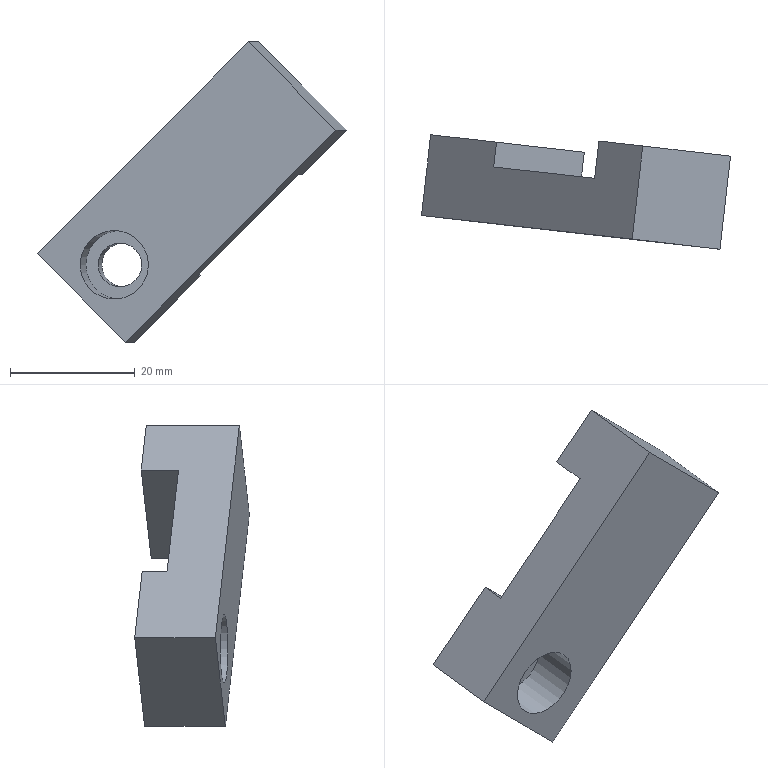Part | NX | features XQ 2 | 1 solid | 13 faces | box 49.472 x 18.36 x 48.083 mm | volume 10087 mm3 | plane 11 | cylinder 2 | commonest cylinder face diameters 7 x1 11 x1
STEP:
#1=CARTESIAN_POINT('',(2718.933,-373.251,-72.883));
#2=VERTEX_POINT('',#1);
#3=CARTESIAN_POINT('',(2735.092,-375.092,-56.62));
#4=VERTEX_POINT('',#3);
#5=CARTESIAN_POINT('',(2735.092,-375.092,-56.62));
#6=DIRECTION('',(0.7026,-0.08005,0.7071));
#7=VECTOR('',#6,1000.);
#8=LINE('',#5,#7);
#9=EDGE_CURVE('',#2,#4,#8,.T.);
#10=ORIENTED_EDGE('',*,*,#9,.F.);
#11=CARTESIAN_POINT('',(2704.882,-371.65,-58.741));
#12=VERTEX_POINT('',#11);
#13=CARTESIAN_POINT('',(2711.907,-372.45,-65.812));
#14=DIRECTION('',(-0.7026,0.08005,0.7071));
#15=VECTOR('',#14,1000.);
#16=LINE('',#13,#15);
#17=EDGE_CURVE('',#2,#12,#16,.T.);
#18=ORIENTED_EDGE('',*,*,#17,.T.);
#19=CARTESIAN_POINT('',(2721.041,-373.491,-42.478));
#20=VERTEX_POINT('',#19);
#21=CARTESIAN_POINT('',(2721.041,-373.491,-42.478));
#22=DIRECTION('',(-0.7026,0.08005,-0.7071));
#23=VECTOR('',#22,1000.);
#24=LINE('',#21,#23);
#25=EDGE_CURVE('',#20,#12,#24,.T.);
#26=ORIENTED_EDGE('',*,*,#25,.F.);
#27=CARTESIAN_POINT('',(2728.066,-374.292,-49.549));
#28=DIRECTION('',(0.7026,-0.08005,-0.7071));
#29=VECTOR('',#28,1000.);
#30=LINE('',#27,#29);
#31=EDGE_CURVE('',#20,#4,#30,.T.);
#32=ORIENTED_EDGE('',*,*,#31,.T.);
#33=EDGE_LOOP('',(#10,#18,#26,#32));
#34=FACE_BOUND('',#33,.T.);
#35=CARTESIAN_POINT('',(2737.38,-375.353,-28.774));
#36=DIRECTION('',(0.1132,0.9936,-0.000000218));
#37=DIRECTION('',(-0.000000616,-0.000000149,-1.));
#38=AXIS2_PLACEMENT_3D('',#35,#36,#37);
#39=PLANE('',#38);
#40=ADVANCED_FACE('',(#34),#39,.T.);
#41=CARTESIAN_POINT('',(2694.796,-366.475,-69.348));
#42=VERTEX_POINT('',#41);
#43=CARTESIAN_POINT('',(2693.325,-379.391,-69.348));
#44=VERTEX_POINT('',#43);
#45=CARTESIAN_POINT('',(2694.457,-369.456,-69.348));
#46=DIRECTION('',(-0.1132,-0.9936,0.000000275));
#47=VECTOR('',#46,1000.);
#48=LINE('',#45,#47);
#49=EDGE_CURVE('',#42,#44,#48,.T.);
#50=ORIENTED_EDGE('',*,*,#49,.F.);
#51=CARTESIAN_POINT('',(2708.847,-368.076,-83.49));
#52=VERTEX_POINT('',#51);
#53=CARTESIAN_POINT('',(2703.578,-367.476,-78.187));
#54=DIRECTION('',(-0.7026,0.08005,0.7071));
#55=VECTOR('',#54,1000.);
#56=LINE('',#53,#55);
#57=EDGE_CURVE('',#52,#42,#56,.T.);
#58=ORIENTED_EDGE('',*,*,#57,.F.);
#59=CARTESIAN_POINT('',(2707.376,-380.992,-83.49));
#60=VERTEX_POINT('',#59);
#61=CARTESIAN_POINT('',(2708.508,-371.057,-83.49));
#62=DIRECTION('',(0.1132,0.9936,-0.000000275));
#63=VECTOR('',#62,1000.);
#64=LINE('',#61,#63);
#65=EDGE_CURVE('',#60,#52,#64,.T.);
#66=ORIENTED_EDGE('',*,*,#65,.F.);
#67=CARTESIAN_POINT('',(2702.107,-380.392,-78.187));
#68=DIRECTION('',(0.7026,-0.08005,-0.7071));
#69=VECTOR('',#68,1000.);
#70=LINE('',#67,#69);
#71=EDGE_CURVE('',#44,#60,#70,.T.);
#72=ORIENTED_EDGE('',*,*,#71,.F.);
#73=EDGE_LOOP('',(#50,#58,#66,#72));
#74=FACE_BOUND('',#73,.T.);
#75=CARTESIAN_POINT('',(2703.239,-370.456,-78.187));
#76=DIRECTION('',(-0.7026,0.08005,-0.7071));
#77=DIRECTION('',(0.7112,0.0435,-0.7017));
#78=AXIS2_PLACEMENT_3D('',#75,#76,#77);
#79=PLANE('',#78);
#80=ADVANCED_FACE('',(#74),#79,.T.);
#81=ORIENTED_EDGE('',*,*,#25,.T.);
#82=CARTESIAN_POINT('',(2705.335,-367.676,-58.741));
#83=VERTEX_POINT('',#82);
#84=CARTESIAN_POINT('',(2704.995,-370.656,-58.741));
#85=DIRECTION('',(0.1132,0.9936,-0.000000275));
#86=VECTOR('',#85,1000.);
#87=LINE('',#84,#86);
#88=EDGE_CURVE('',#12,#83,#87,.T.);
#89=ORIENTED_EDGE('',*,*,#88,.T.);
#90=CARTESIAN_POINT('',(2721.493,-369.517,-42.478));
#91=DIRECTION('',(-0.7026,0.08005,-0.7071));
#92=VECTOR('',#91,1000.);
#93=LINE('',#90,#92);
#94=EDGE_CURVE('',#83,#42,#93,.T.);
#95=ORIENTED_EDGE('',*,*,#94,.T.);
#96=ORIENTED_EDGE('',*,*,#49,.T.);
#97=CARTESIAN_POINT('',(2727.047,-383.234,-35.407));
#98=VERTEX_POINT('',#97);
#99=CARTESIAN_POINT('',(2720.022,-382.433,-42.478));
#100=DIRECTION('',(-0.7026,0.08005,-0.7071));
#101=VECTOR('',#100,1000.);
#102=LINE('',#99,#101);
#103=EDGE_CURVE('',#98,#44,#102,.T.);
#104=ORIENTED_EDGE('',*,*,#103,.F.);
#105=CARTESIAN_POINT('',(2728.745,-368.33,-35.407));
#106=VERTEX_POINT('',#105);
#107=CARTESIAN_POINT('',(2728.179,-373.298,-35.407));
#108=DIRECTION('',(0.1132,0.9936,-0.000000275));
#109=VECTOR('',#108,1000.);
#110=LINE('',#107,#109);
#111=EDGE_CURVE('',#98,#106,#110,.T.);
#112=ORIENTED_EDGE('',*,*,#111,.T.);
#113=CARTESIAN_POINT('',(2721.72,-367.53,-42.478));
#114=VERTEX_POINT('',#113);
#115=CARTESIAN_POINT('',(2714.694,-366.729,-49.549));
#116=DIRECTION('',(-0.7026,0.08005,-0.7071));
#117=VECTOR('',#116,1000.);
#118=LINE('',#115,#117);
#119=EDGE_CURVE('',#106,#114,#118,.T.);
#120=ORIENTED_EDGE('',*,*,#119,.T.);
#121=CARTESIAN_POINT('',(2721.154,-372.498,-42.478));
#122=DIRECTION('',(0.1132,0.9936,-0.000000275));
#123=VECTOR('',#122,1000.);
#124=LINE('',#121,#123);
#125=EDGE_CURVE('',#20,#114,#124,.T.);
#126=ORIENTED_EDGE('',*,*,#125,.F.);
#127=EDGE_LOOP('',(#81,#89,#95,#96,#104,#112,#120,#126));
#128=FACE_BOUND('',#127,.T.);
#129=CARTESIAN_POINT('',(2721.154,-372.498,-42.478));
#130=DIRECTION('',(-0.7026,0.08005,0.7071));
#131=DIRECTION('',(-0.6832,0.2024,-0.7017));
#132=AXIS2_PLACEMENT_3D('',#129,#130,#131);
#133=PLANE('',#132);
#134=ADVANCED_FACE('',(#128),#133,.T.);
#135=ORIENTED_EDGE('',*,*,#9,.T.);
#136=CARTESIAN_POINT('',(2735.771,-369.131,-56.62));
#137=VERTEX_POINT('',#136);
#138=CARTESIAN_POINT('',(2735.205,-374.098,-56.62));
#139=DIRECTION('',(0.1132,0.9936,-0.000000275));
#140=VECTOR('',#139,1000.);
#141=LINE('',#138,#140);
#142=EDGE_CURVE('',#4,#137,#141,.T.);
#143=ORIENTED_EDGE('',*,*,#142,.T.);
#144=CARTESIAN_POINT('',(2742.797,-369.931,-49.549));
#145=VERTEX_POINT('',#144);
#146=CARTESIAN_POINT('',(2728.745,-368.33,-63.691));
#147=DIRECTION('',(-0.7026,0.08005,-0.7071));
#148=VECTOR('',#147,1000.);
#149=LINE('',#146,#148);
#150=EDGE_CURVE('',#145,#137,#149,.T.);
#151=ORIENTED_EDGE('',*,*,#150,.F.);
#152=CARTESIAN_POINT('',(2741.099,-384.835,-49.549));
#153=VERTEX_POINT('',#152);
#154=CARTESIAN_POINT('',(2742.231,-374.899,-49.549));
#155=DIRECTION('',(-0.1132,-0.9936,0.000000275));
#156=VECTOR('',#155,1000.);
#157=LINE('',#154,#156);
#158=EDGE_CURVE('',#145,#153,#157,.T.);
#159=ORIENTED_EDGE('',*,*,#158,.T.);
#160=CARTESIAN_POINT('',(2734.073,-384.034,-56.62));
#161=DIRECTION('',(-0.7026,0.08005,-0.7071));
#162=VECTOR('',#161,1000.);
#163=LINE('',#160,#162);
#164=EDGE_CURVE('',#153,#60,#163,.T.);
#165=ORIENTED_EDGE('',*,*,#164,.T.);
#166=ORIENTED_EDGE('',*,*,#65,.T.);
#167=CARTESIAN_POINT('',(2719.386,-369.277,-72.883));
#168=VERTEX_POINT('',#167);
#169=CARTESIAN_POINT('',(2735.545,-371.118,-56.62));
#170=DIRECTION('',(-0.7026,0.08005,-0.7071));
#171=VECTOR('',#170,1000.);
#172=LINE('',#169,#171);
#173=EDGE_CURVE('',#168,#52,#172,.T.);
#174=ORIENTED_EDGE('',*,*,#173,.F.);
#175=CARTESIAN_POINT('',(2719.046,-372.257,-72.883));
#176=DIRECTION('',(0.1132,0.9936,-0.000000275));
#177=VECTOR('',#176,1000.);
#178=LINE('',#175,#177);
#179=EDGE_CURVE('',#2,#168,#178,.T.);
#180=ORIENTED_EDGE('',*,*,#179,.F.);
#181=EDGE_LOOP('',(#135,#143,#151,#159,#165,#166,#174,#180));
#182=FACE_BOUND('',#181,.T.);
#183=CARTESIAN_POINT('',(2735.205,-374.098,-56.62));
#184=DIRECTION('',(0.7026,-0.08005,-0.7071));
#185=DIRECTION('',(0.6832,-0.2024,0.7017));
#186=AXIS2_PLACEMENT_3D('',#183,#184,#185);
#187=PLANE('',#186);
#188=ADVANCED_FACE('',(#182),#187,.T.);
#189=ORIENTED_EDGE('',*,*,#158,.F.);
#190=CARTESIAN_POINT('',(2737.527,-369.331,-44.246));
#191=DIRECTION('',(0.7026,-0.08005,-0.7071));
#192=VECTOR('',#191,1000.);
#193=LINE('',#190,#192);
#194=EDGE_CURVE('',#106,#145,#193,.T.);
#195=ORIENTED_EDGE('',*,*,#194,.F.);
#196=ORIENTED_EDGE('',*,*,#111,.F.);
#197=CARTESIAN_POINT('',(2735.829,-384.234,-44.246));
#198=DIRECTION('',(-0.7026,0.08005,0.7071));
#199=VECTOR('',#198,1000.);
#200=LINE('',#197,#199);
#201=EDGE_CURVE('',#153,#98,#200,.T.);
#202=ORIENTED_EDGE('',*,*,#201,.F.);
#203=EDGE_LOOP('',(#189,#195,#196,#202));
#204=FACE_BOUND('',#203,.T.);
#205=CARTESIAN_POINT('',(2736.961,-374.299,-44.246));
#206=DIRECTION('',(0.7026,-0.08005,0.7071));
#207=DIRECTION('',(-0.7112,-0.0435,0.7017));
#208=AXIS2_PLACEMENT_3D('',#205,#206,#207);
#209=PLANE('',#208);
#210=ADVANCED_FACE('',(#204),#209,.T.);
#211=ORIENTED_EDGE('',*,*,#103,.T.);
#212=ORIENTED_EDGE('',*,*,#71,.T.);
#213=ORIENTED_EDGE('',*,*,#164,.F.);
#214=ORIENTED_EDGE('',*,*,#201,.T.);
#215=EDGE_LOOP('',(#211,#212,#213,#214));
#216=FACE_BOUND('',#215,.T.);
#217=CARTESIAN_POINT('',(2711.084,-381.415,-71.116));
#218=VERTEX_POINT('',#217);
#219=CARTESIAN_POINT('',(2705.619,-380.792,-71.116));
#220=DIRECTION('',(0.1132,0.9936,-0.000000275));
#221=DIRECTION('',(0.9936,-0.1132,0.));
#222=AXIS2_PLACEMENT_3D('',#219,#220,#221);
#223=CIRCLE('',#222,5.5);
#224=EDGE_CURVE('',#218,#218,#223,.T.);
#225=ORIENTED_EDGE('',*,*,#224,.T.);
#226=EDGE_LOOP('',(#225));
#227=FACE_BOUND('',#226,.T.);
#228=CARTESIAN_POINT('',(2725.291,-383.034,-47.781));
#229=DIRECTION('',(-0.1132,-0.9936,0.000000275));
#230=DIRECTION('',(0.000000623,0.000000206,1.));
#231=AXIS2_PLACEMENT_3D('',#228,#229,#230);
#232=PLANE('',#231);
#233=ADVANCED_FACE('',(#216,#227),#232,.T.);
#234=CARTESIAN_POINT('',(2711.99,-373.466,-71.116));
#235=VERTEX_POINT('',#234);
#236=CARTESIAN_POINT('',(2706.525,-372.844,-71.116));
#237=DIRECTION('',(0.1132,0.9936,-0.000000275));
#238=DIRECTION('',(0.9936,-0.1132,0.));
#239=AXIS2_PLACEMENT_3D('',#236,#237,#238);
#240=CIRCLE('',#239,5.5);
#241=EDGE_CURVE('',#235,#235,#240,.T.);
#242=ORIENTED_EDGE('',*,*,#241,.T.);
#243=EDGE_LOOP('',(#242));
#244=FACE_BOUND('',#243,.T.);
#245=ORIENTED_EDGE('',*,*,#224,.F.);
#246=EDGE_LOOP('',(#245));
#247=FACE_BOUND('',#246,.T.);
#248=CARTESIAN_POINT('',(2706.185,-375.824,-71.116));
#249=DIRECTION('',(0.1132,0.9936,-0.000000275));
#250=DIRECTION('',(0.1725,-0.01966,-0.9848));
#251=AXIS2_PLACEMENT_3D('',#248,#249,#250);
#252=CYLINDRICAL_SURFACE('',#251,5.5);
#253=ADVANCED_FACE('',(#244,#247),#252,.F.);
#254=CARTESIAN_POINT('',(2710.002,-373.24,-71.116));
#255=VERTEX_POINT('',#254);
#256=CARTESIAN_POINT('',(2706.525,-372.844,-71.116));
#257=DIRECTION('',(-0.1132,-0.9936,0.000000275));
#258=DIRECTION('',(0.9936,-0.1132,0.));
#259=AXIS2_PLACEMENT_3D('',#256,#257,#258);
#260=CIRCLE('',#259,3.5);
#261=EDGE_CURVE('',#255,#255,#260,.T.);
#262=ORIENTED_EDGE('',*,*,#261,.F.);
#263=EDGE_LOOP('',(#262));
#264=FACE_BOUND('',#263,.T.);
#265=ORIENTED_EDGE('',*,*,#241,.F.);
#266=EDGE_LOOP('',(#265));
#267=FACE_BOUND('',#266,.T.);
#268=CARTESIAN_POINT('',(2706.525,-372.844,-71.116));
#269=DIRECTION('',(-0.1132,-0.9936,0.000000275));
#270=DIRECTION('',(0.000000623,0.000000206,1.));
#271=AXIS2_PLACEMENT_3D('',#268,#269,#270);
#272=PLANE('',#271);
#273=ADVANCED_FACE('',(#264,#267),#272,.T.);
#274=ORIENTED_EDGE('',*,*,#17,.F.);
#275=ORIENTED_EDGE('',*,*,#179,.T.);
#276=CARTESIAN_POINT('',(2712.36,-368.476,-65.812));
#277=DIRECTION('',(-0.7026,0.08005,0.7071));
#278=VECTOR('',#277,1000.);
#279=LINE('',#276,#278);
#280=EDGE_CURVE('',#168,#83,#279,.T.);
#281=ORIENTED_EDGE('',*,*,#280,.T.);
#282=ORIENTED_EDGE('',*,*,#88,.F.);
#283=EDGE_LOOP('',(#274,#275,#281,#282));
#284=FACE_BOUND('',#283,.T.);
#285=CARTESIAN_POINT('',(2712.021,-371.457,-65.812));
#286=DIRECTION('',(0.7026,-0.08005,0.7071));
#287=DIRECTION('',(-0.7112,-0.0435,0.7017));
#288=AXIS2_PLACEMENT_3D('',#285,#286,#287);
#289=PLANE('',#288);
#290=ADVANCED_FACE('',(#284),#289,.T.);
#291=CARTESIAN_POINT('',(2703.613,-367.48,-71.116));
#292=VERTEX_POINT('',#291);
#293=CARTESIAN_POINT('',(2707.091,-367.876,-71.116));
#294=DIRECTION('',(0.1132,0.9936,-0.000000275));
#295=DIRECTION('',(-0.9936,0.1132,0.));
#296=AXIS2_PLACEMENT_3D('',#293,#294,#295);
#297=CIRCLE('',#296,3.5);
#298=EDGE_CURVE('',#292,#292,#297,.T.);
#299=ORIENTED_EDGE('',*,*,#298,.F.);
#300=EDGE_LOOP('',(#299));
#301=FACE_BOUND('',#300,.T.);
#302=ORIENTED_EDGE('',*,*,#94,.F.);
#303=ORIENTED_EDGE('',*,*,#280,.F.);
#304=ORIENTED_EDGE('',*,*,#173,.T.);
#305=ORIENTED_EDGE('',*,*,#57,.T.);
#306=EDGE_LOOP('',(#302,#303,#304,#305));
#307=FACE_BOUND('',#306,.T.);
#308=CARTESIAN_POINT('',(2730.275,-370.517,-51.317));
#309=DIRECTION('',(0.1132,0.9936,-0.000000275));
#310=DIRECTION('',(-0.000000623,-0.000000206,-1.));
#311=AXIS2_PLACEMENT_3D('',#308,#309,#310);
#312=PLANE('',#311);
#313=ADVANCED_FACE('',(#301,#307),#312,.T.);
#314=ORIENTED_EDGE('',*,*,#298,.T.);
#315=EDGE_LOOP('',(#314));
#316=FACE_BOUND('',#315,.T.);
#317=ORIENTED_EDGE('',*,*,#261,.T.);
#318=EDGE_LOOP('',(#317));
#319=FACE_BOUND('',#318,.T.);
#320=CARTESIAN_POINT('',(2706.185,-375.824,-71.116));
#321=DIRECTION('',(0.1132,0.9936,-0.000000275));
#322=DIRECTION('',(0.1725,-0.01966,-0.9848));
#323=AXIS2_PLACEMENT_3D('',#320,#321,#322);
#324=CYLINDRICAL_SURFACE('',#323,3.5);
#325=ADVANCED_FACE('',(#316,#319),#324,.F.);
#326=ORIENTED_EDGE('',*,*,#31,.F.);
#327=ORIENTED_EDGE('',*,*,#125,.T.);
#328=CARTESIAN_POINT('',(2730.502,-368.53,-51.317));
#329=DIRECTION('',(-0.7026,0.08005,0.7071));
#330=VECTOR('',#329,1000.);
#331=LINE('',#328,#330);
#332=EDGE_CURVE('',#137,#114,#331,.T.);
#333=ORIENTED_EDGE('',*,*,#332,.F.);
#334=ORIENTED_EDGE('',*,*,#142,.F.);
#335=EDGE_LOOP('',(#326,#327,#333,#334));
#336=FACE_BOUND('',#335,.T.);
#337=CARTESIAN_POINT('',(2728.179,-373.298,-49.549));
#338=DIRECTION('',(-0.7026,0.08005,-0.7071));
#339=DIRECTION('',(0.7112,0.0435,-0.7017));
#340=AXIS2_PLACEMENT_3D('',#337,#338,#339);
#341=PLANE('',#340);
#342=ADVANCED_FACE('',(#336),#341,.T.);
#343=ORIENTED_EDGE('',*,*,#150,.T.);
#344=ORIENTED_EDGE('',*,*,#332,.T.);
#345=ORIENTED_EDGE('',*,*,#119,.F.);
#346=ORIENTED_EDGE('',*,*,#194,.T.);
#347=EDGE_LOOP('',(#343,#344,#345,#346));
#348=FACE_BOUND('',#347,.T.);
#349=CARTESIAN_POINT('',(2723.476,-367.73,-58.388));
#350=DIRECTION('',(0.1132,0.9936,-0.000000275));
#351=DIRECTION('',(-0.000000623,-0.000000206,-1.));
#352=AXIS2_PLACEMENT_3D('',#349,#350,#351);
#353=PLANE('',#352);
#354=ADVANCED_FACE('',(#348),#353,.T.);
#355=CLOSED_SHELL('',(#40,#80,#134,#188,#210,#233,#253,#273,#290,#313,#325,#342,#354));
#356=MANIFOLD_SOLID_BREP('',#355);
#357=(LENGTH_UNIT()NAMED_UNIT(*)SI_UNIT(.MILLI.,.METRE.));
#358=UNCERTAINTY_MEASURE_WITH_UNIT(LENGTH_MEASURE(0.00001),#357,'','');
#359=(NAMED_UNIT(*)PLANE_ANGLE_UNIT()SI_UNIT($,.RADIAN.));
#360=(NAMED_UNIT(*)SI_UNIT($,.STERADIAN.)SOLID_ANGLE_UNIT());
#361=(GEOMETRIC_REPRESENTATION_CONTEXT(3)GLOBAL_UNCERTAINTY_ASSIGNED_CONTEXT((#358))GLOBAL_UNIT_ASSIGNED_CONTEXT((#357,#359,#360))REPRESENTATION_CONTEXT('',''));
#362=ADVANCED_BREP_SHAPE_REPRESENTATION('',(#356),#361);